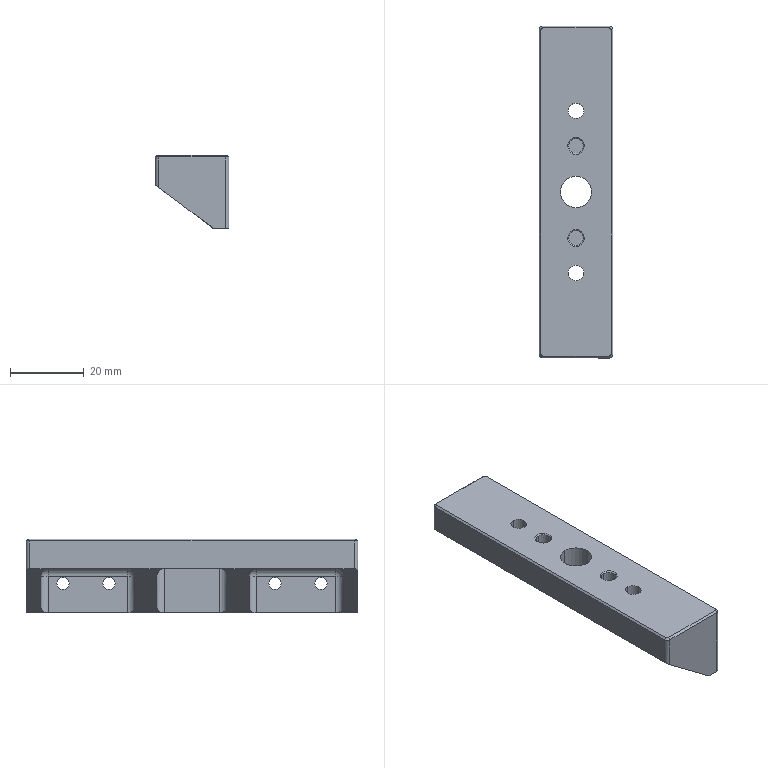NC program | NX | posted with a generic post | part box 20 x 90 x 20 mm
Lines 987 to 2039 of 22268:
(FIXED_CONTOUR , TOOL : D4R0.5)
N1966 T18 M6
N1968 G54
N1970 G17 G0 G90 X37.898 Y-9.972 B0. C0. S9500 M3
N1972 G43 Z30. H18
N1974 Z-7.6
N1976 G94 G1 Z-11.96 F1000.
N1978 X37.887 Y-9.944
N1980 X37.86 Y-9.928
N1982 X37.829 Y-9.932
N1984 X37.745 Z-11.98 F2500.
N1986 X37.579 Z-11.997
N1988 X37.321 Z-12.
N1990 X18.997 Z-11.999
N1992 X18.898 Z-11.996
N1994 X18.751 Z-11.979
N1996 X18.69 Z-11.965
N1998 X18.547 Y-9.858 Z-11.931
N2000 X18.751 Z-11.979
N2002 X18.933 Z-11.998
N2004 X19.144 Z-12.
N2006 X37.53 Y-9.859 Z-11.999
N2008 X37.568 Z-11.998
N2010 X37.745 Z-11.98
N2012 X37.955 Z-11.93
N2014 X37.995 Y-9.835 Z-11.917
N2016 X38.034 Y-9.811 Z-11.9
N2018 X38.082 Y-9.775 Z-11.879
N2020 X37.943 Z-11.933
N2022 X37.745 Z-11.98
N2024 X37.553 Z-11.998
N2026 X37.459 Z-12.
N2028 X19.026
N2030 X18.938 Z-11.998
N2032 X18.751 Z-11.979
N2034 X18.553 Z-11.932
N2036 X18.418 Z-11.879
N2038 X18.356 Y-9.73 Z-11.852
N2040 X18.317 Y-9.702 Z-11.831
N2042 X18.301 Y-9.687 Z-11.822
N2044 X18.355 Z-11.851
N2046 X18.553 Z-11.931
N2048 X18.751 Z-11.978
N2050 X18.949 Z-11.999
N2052 X19.048 Z-12.
N2054 X37.498 Y-9.688
N2056 X37.547 Z-11.998
N2058 X37.745 Z-11.979
N2060 X37.943 Z-11.932
N2062 X38.141 Z-11.854
N2064 X38.194 Z-11.825
N2066 X38.231 Y-9.658 Z-11.805
N2068 X38.288 Y-9.593 Z-11.774
N2070 X38.141 Z-11.853
N2072 X37.943 Z-11.932
N2074 X37.745 Z-11.979
N2076 X37.547 Z-11.998
N2078 X37.498 Z-12.
N2080 X19.048
N2082 X18.949 Z-11.999
N2084 X18.751 Z-11.978
N2086 X18.553 Z-11.931
N2088 X18.355 Z-11.851
N2090 X18.213 Z-11.773
N2092 X18.157 Y-9.529 Z-11.743
N2094 X18.13 Y-9.497 Z-11.725
N2096 X18.157 Z-11.743
N2098 X18.355 Z-11.851
N2100 X18.553 Z-11.931
N2102 X18.751 Z-11.978
N2104 X18.949 Z-11.999
N2106 X19.048 Z-12.
N2108 X37.498
N2110 X37.547 Z-11.998
N2112 X37.745 Z-11.979
N2114 X37.943 Z-11.932
N2116 X38.141 Z-11.853
N2118 X38.339 Z-11.745
N2120 X38.368 Z-11.722
N2122 X38.39 Y-9.468 Z-11.704
N2124 X38.438 Y-9.4 Z-11.665
N2126 X38.339 Z-11.744
N2128 X38.141 Z-11.853
N2130 X37.943 Z-11.932
N2132 X37.745 Z-11.979
N2134 X37.547 Z-11.998
N2136 X37.498 Z-12.
N2138 X19.048
N2140 X18.949 Z-11.999
N2142 X18.751 Z-11.978
N2144 X18.553 Z-11.931
N2146 X18.355 Z-11.851
N2148 X18.157 Z-11.742
N2150 X18.125 Z-11.72
N2152 X18.06 Z-11.668
N2154 X18.017 Y-9.334 Z-11.627
N2156 X17.995 Y-9.303 Z-11.609
N2158 X18.157 Z-11.741
N2160 X18.355 Z-11.851
N2162 X18.553 Z-11.931
N2164 X18.751 Z-11.978
N2166 X18.949 Z-11.999
N2168 X19.048 Z-12.
N2170 X37.498
N2172 X37.547 Z-11.998
N2174 X37.745 Z-11.979
N2176 X37.943 Z-11.932
N2178 X38.141 Z-11.853
N2180 X38.339 Z-11.743
N2182 X38.505 Z-11.61
N2184 X38.537 Y-9.257 Z-11.584
N2186 X38.564 Y-9.205 Z-11.555
N2188 X38.537 Z-11.584
N2190 X38.339 Z-11.743
N2192 X38.141 Z-11.853
N2194 X37.943 Z-11.932
N2196 X37.745 Z-11.979
N2198 X37.547 Z-11.998
N2200 X37.498 Z-12.
N2202 X19.048
N2204 X18.949 Z-11.999
N2206 X18.751 Z-11.978
N2208 X18.553 Z-11.931
N2210 X18.355 Z-11.851
N2212 X18.157 Z-11.741
N2214 X17.96 Z-11.58
N2216 X17.934 Z-11.553
N2218 X17.92 Y-9.178 Z-11.537
N2220 X17.886 Y-9.107 Z-11.499
N2222 X17.96 Z-11.58
N2224 X18.101 Z-11.697
N2226 X18.157 Z-11.741
N2228 X18.355 Z-11.851
N2230 X18.553 Z-11.931
N2232 X18.751 Z-11.978
N2234 X18.949 Z-11.999
N2236 X19.048 Z-12.
N2238 X37.498
N2240 X37.547 Z-11.998
N2242 X37.745 Z-11.979
N2244 X37.943 Z-11.932
N2246 X38.141 Z-11.853
N2248 X38.339 Z-11.743
N2250 X38.396 Z-11.699
N2252 X38.537 Z-11.584
N2254 X38.616 Z-11.498
N2256 X38.664 Y-9.009 Z-11.446
N2258 X38.537 Z-11.584
N2260 X38.42 Z-11.68
N2262 X38.339 Z-11.743
N2264 X38.141 Z-11.853
N2266 X37.943 Z-11.932
N2268 X37.745 Z-11.979
N2270 X37.547 Z-11.998
N2272 X37.498 Z-12.
N2274 X19.048
N2276 X18.949 Z-11.999
N2278 X18.751 Z-11.978
N2280 X18.553 Z-11.931
N2282 X18.355 Z-11.851
N2284 X18.157 Z-11.741
N2286 X18.076 Z-11.678
N2288 X17.96 Z-11.579
N2290 X17.838 Z-11.447
N2292 X17.796 Y-8.91 Z-11.391
N2294 X17.861 Z-11.472
N2296 X17.96 Z-11.579
N2298 X18.059 Z-11.664
N2300 X18.157 Z-11.741
N2302 X18.355 Z-11.851
N2304 X18.553 Z-11.931
N2306 X18.751 Z-11.978
N2308 X18.949 Z-11.999
N2310 X19.048 Z-12.
N2312 X37.498
N2314 X37.547 Z-11.998
N2316 X37.745 Z-11.979
N2318 X37.943 Z-11.932
N2320 X38.141 Z-11.853
N2322 X38.339 Z-11.743
N2324 X38.438 Z-11.667
N2326 X38.537 Z-11.583
N2328 X38.643 Z-11.469
N2330 X38.705 Z-11.388
N2332 X38.745 Y-8.811 Z-11.333
N2334 X38.735 Z-11.349
N2336 X38.636 Z-11.478
N2338 X38.537 Z-11.583
N2340 X38.438 Z-11.667
N2342 X38.339 Z-11.743
N2344 X38.141 Z-11.853
N2346 X37.943 Z-11.932
N2348 X37.745 Z-11.979
N2350 X37.547 Z-11.998
N2352 X37.498 Z-12.
N2354 X19.048
N2356 X18.949 Z-11.999
N2358 X18.751 Z-11.978
N2360 X18.553 Z-11.931
N2362 X18.355 Z-11.851
N2364 X18.157 Z-11.741
N2366 X18.059 Z-11.664
N2368 X17.96 Z-11.579
N2370 X17.861 Z-11.472
N2372 X17.762 Z-11.347
N2374 X17.756 Z-11.337
N2376 X17.722 Y-8.712 Z-11.282
N2378 X17.762 Z-11.347
N2380 X17.861 Z-11.472
N2382 X17.96 Z-11.579
N2384 X18.059 Z-11.664
N2386 X18.157 Z-11.741
N2388 X18.355 Z-11.851
N2390 X18.553 Z-11.931
N2392 X18.751 Z-11.978
N2394 X18.949 Z-11.999
N2396 X19.048 Z-12.
N2398 X37.498
N2400 X37.547 Z-11.998
N2402 X37.745 Z-11.979
N2404 X37.943 Z-11.932
N2406 X38.141 Z-11.853
N2408 X38.339 Z-11.743
N2410 X38.438 Z-11.667
N2412 X38.537 Z-11.583
N2414 X38.636 Z-11.478
N2416 X38.735 Z-11.349
N2418 X38.779 Z-11.276
N2420 X38.811 Y-8.613 Z-11.221
N2422 X38.735 Z-11.349
N2424 X38.636 Z-11.478
N2426 X38.537 Z-11.583
N2428 X38.438 Z-11.667
N2430 X38.339 Z-11.743
N2432 X38.141 Z-11.853
N2434 X37.943 Z-11.932
N2436 X37.745 Z-11.979
N2438 X37.547 Z-11.998
N2440 X37.498 Z-12.
N2442 X19.048
N2444 X18.949 Z-11.999
N2446 X18.751 Z-11.978
N2448 X18.553 Z-11.931
N2450 X18.355 Z-11.851
N2452 X18.157 Z-11.741
N2454 X18.059 Z-11.664
N2456 X17.96 Z-11.579
N2458 X17.861 Z-11.472
N2460 X17.762 Z-11.346
N2462 X17.691 Z-11.225
N2464 X17.66 Y-8.514 Z-11.169
N2466 X17.762 Z-11.346
N2468 X17.861 Z-11.472
N2470 X17.96 Z-11.579
N2472 X18.059 Z-11.664
N2474 X18.157 Z-11.741
N2476 X18.355 Z-11.851
N2478 X18.553 Z-11.931
N2480 X18.751 Z-11.978
N2482 X18.949 Z-11.999
N2484 X19.048 Z-12.
N2486 X37.498 Y-8.515
N2488 X37.547 Z-11.998
N2490 X37.745 Z-11.979
N2492 X37.943 Z-11.932
N2494 X38.141 Z-11.853
N2496 X38.339 Z-11.743
N2498 X38.438 Z-11.667
N2500 X38.537 Z-11.583
N2502 X38.636 Z-11.478
N2504 X38.735 Z-11.349
N2506 X38.841 Z-11.166
N2508 X38.869 Y-8.416 Z-11.113
N2510 X38.834 Z-11.181
N2512 X38.735 Z-11.349
N2514 X38.636 Z-11.478
N2516 X38.537 Z-11.583
N2518 X38.438 Z-11.667
N2520 X38.339 Z-11.743
N2522 X38.141 Z-11.853
N2524 X37.943 Z-11.932
N2526 X37.745 Z-11.979
N2528 X37.547 Z-11.998
N2530 X37.498 Z-12.
N2532 X19.048 Y-8.415
N2534 X18.949 Z-11.999
N2536 X18.751 Z-11.978
N2538 X18.553 Z-11.931
N2540 X18.355 Z-11.851
N2542 X18.157 Z-11.741
N2544 X18.059 Z-11.664
N2546 X17.96 Z-11.579
N2548 X17.861 Z-11.472
N2550 X17.762 Z-11.346
N2552 X17.663 Z-11.174
N2554 X17.632 Z-11.114
N2556 X17.605 Y-8.316 Z-11.061
N2558 X17.635 Z-11.115
N2560 X17.663 Z-11.174
N2562 X17.762 Z-11.346
N2564 X17.861 Z-11.472
N2566 X17.96 Z-11.579
N2568 X18.059 Z-11.664
N2570 X18.157 Z-11.741
N2572 X18.355 Z-11.851
N2574 X18.553 Z-11.931
N2576 X18.751 Z-11.978
N2578 X18.949 Z-11.999
N2580 X19.048 Z-12.
N2582 X37.498
N2584 X37.547 Z-11.998
N2586 X37.745 Z-11.979
N2588 X37.943 Z-11.932
N2590 X38.141 Z-11.853
N2592 X38.339 Z-11.743
N2594 X38.438 Z-11.667
N2596 X38.537 Z-11.583
N2598 X38.636 Z-11.478
N2600 X38.735 Z-11.349
N2602 X38.834 Z-11.181
N2604 X38.862 Z-11.123
N2606 X38.896 Z-11.06
N2608 X38.902 Y-8.296 Z-11.049
N2610 X38.913 Y-8.218 Z-11.002
N2612 X38.892 Z-11.065
N2614 X38.834 Z-11.181
N2616 X38.735 Z-11.349
N2618 X38.636 Z-11.478
N2620 X38.537 Z-11.583
N2622 X38.438 Z-11.667
N2624 X38.339 Z-11.743
N2626 X38.141 Z-11.853
N2628 X37.943 Z-11.932
N2630 X37.745 Z-11.979
N2632 X37.547 Z-11.998
N2634 X37.498 Z-12.
N2636 X19.048
N2638 X18.949 Z-11.999
N2640 X18.751 Z-11.978
N2642 X18.553 Z-11.931
N2644 X18.355 Z-11.851
N2646 X18.157 Z-11.741
N2648 X18.059 Z-11.664
N2650 X17.96 Z-11.579
N2652 X17.861 Z-11.472
N2654 X17.762 Z-11.346
N2656 X17.663 Z-11.174
N2658 X17.622 Z-11.089
N2660 X17.604 Z-11.056
N2662 X17.587 Z-11.002
N2664 X17.571 Y-8.118 Z-10.944
N2666 X17.613 Z-11.071
N2668 X17.663 Z-11.174
N2670 X17.762 Z-11.346
N2672 X17.861 Z-11.472
N2674 X17.96 Z-11.579
N2676 X18.059 Z-11.664
N2678 X18.157 Z-11.741
N2680 X18.355 Z-11.851
N2682 X18.553 Z-11.931
N2684 X18.751 Z-11.978
N2686 X18.949 Z-11.999
N2688 X19.048 Z-12.
N2690 X37.498 Y-8.119
N2692 X37.547 Z-11.998
N2694 X37.745 Z-11.979
N2696 X37.943 Z-11.931
N2698 X38.141 Z-11.853
N2700 X38.339 Z-11.743
N2702 X38.438 Z-11.667
N2704 X38.537 Z-11.583
N2706 X38.636 Z-11.478
N2708 X38.735 Z-11.349
N2710 X38.834 Z-11.181
N2712 X38.883 Z-11.079
N2714 X38.93 Z-10.945
N2716 X38.949 Y-8.019 Z-10.888
N2718 X38.883 Z-11.079
N2720 X38.834 Z-11.181
N2722 X38.735 Z-11.349
N2724 X38.636 Z-11.478
N2726 X38.537 Z-11.583
N2728 X38.438 Z-11.667
N2730 X38.339 Z-11.743
N2732 X38.141 Z-11.853
N2734 X37.943 Z-11.931
N2736 X37.745 Z-11.979
N2738 X37.547 Z-11.998
N2740 X37.498 Z-12.
N2742 X19.048
N2744 X18.949 Z-11.999
N2746 X18.751 Z-11.978
N2748 X18.553 Z-11.931
N2750 X18.355 Z-11.851
N2752 X18.157 Z-11.741
N2754 X18.059 Z-11.664
N2756 X17.96 Z-11.579
N2758 X17.861 Z-11.472
N2760 X17.762 Z-11.345
N2762 X17.663 Z-11.174
N2764 X17.613 Z-11.071
N2766 X17.564 Z-10.924
N2768 X17.555 Z-10.888
N2770 X17.541 Y-7.92 Z-10.832
N2772 X17.564 Z-10.923
N2774 X17.613 Z-11.071
N2776 X17.663 Z-11.174
N2778 X17.762 Z-11.345
N2780 X17.861 Z-11.472
N2782 X17.96 Z-11.579
N2784 X18.059 Z-11.663
N2786 X18.157 Z-11.741
N2788 X18.355 Z-11.851
N2790 X18.553 Z-11.931
N2792 X18.751 Z-11.978
N2794 X18.949 Z-11.999
N2796 X19.048 Z-12.
N2798 X37.498
N2800 X37.547 Z-11.998
N2802 X37.745 Z-11.978
N2804 X37.943 Z-11.931
N2806 X38.141 Z-11.853
N2808 X38.339 Z-11.743
N2810 X38.438 Z-11.667
N2812 X38.537 Z-11.583
N2814 X38.636 Z-11.478
N2816 X38.735 Z-11.349
N2818 X38.834 Z-11.181
N2820 X38.883 Z-11.079
N2822 X38.954 Z-10.874
N2824 X38.963 Z-10.829
N2826 X38.972 Y-7.82 Z-10.769
N2828 X38.941 Z-10.91
N2830 X38.883 Z-11.079
N2832 X38.834 Z-11.181
N2834 X38.735 Z-11.349
N2836 X38.636 Z-11.478
N2838 X38.537 Z-11.583
N2840 X38.438 Z-11.667
N2842 X38.339 Z-11.743
N2844 X38.141 Z-11.853
N2846 X37.943 Z-11.931
N2848 X37.745 Z-11.978
N2850 X37.547 Z-11.998
N2852 X37.498 Z-12.
N2854 X19.048
N2856 X18.949 Z-11.999
N2858 X18.751 Z-11.978
N2860 X18.553 Z-11.931
N2862 X18.355 Z-11.851
N2864 X18.157 Z-11.741
N2866 X18.059 Z-11.663
N2868 X17.96 Z-11.579
N2870 X17.861 Z-11.472
N2872 X17.762 Z-11.345
N2874 X17.663 Z-11.174
N2876 X17.613 Z-11.071
N2878 X17.564 Z-10.923
N2880 X17.53 Z-10.775
N2882 X17.518 Y-7.72 Z-10.718
N2884 X17.564 Z-10.923
N2886 X17.613 Z-11.071
N2888 X17.663 Z-11.174
N2890 X17.762 Z-11.345
N2892 X17.861 Z-11.472
N2894 X17.96 Z-11.579
N2896 X18.059 Z-11.663
N2898 X18.157 Z-11.741
N2900 X18.355 Z-11.851
N2902 X18.553 Z-11.931
N2904 X18.751 Z-11.978
N2906 X18.949 Z-11.999
N2908 X19.048 Z-12.
N2910 X37.498 Y-7.721
N2912 X37.547 Z-11.998
N2914 X37.745 Z-11.978
N2916 X37.943 Z-11.931
N2918 X38.141 Z-11.853
N2920 X38.339 Z-11.743
N2922 X38.438 Z-11.667
N2924 X38.537 Z-11.583
N2926 X38.636 Z-11.478
N2928 X38.735 Z-11.349
N2930 X38.834 Z-11.181
N2932 X38.883 Z-11.079
N2934 X38.933 Z-10.935
N2936 X38.982 Z-10.709
N2938 X38.985 Y-7.681 Z-10.684
N2940 X38.988 Y-7.622 Z-10.643
N2942 X38.982 Z-10.707
N2944 X38.933 Z-10.935
N2946 X38.883 Z-11.079
N2948 X38.834 Z-11.181
N2950 X38.735 Z-11.349
N2952 X38.636 Z-11.478
N2954 X38.537 Z-11.583
N2956 X38.438 Z-11.667
N2958 X38.339 Y-7.621 Z-11.743
N2960 X38.141 Z-11.853
N2962 X37.943 Z-11.931
N2964 X37.745 Z-11.978
N2966 X37.547 Z-11.998
N2968 X37.498 Z-12.
N2970 X19.048
N2972 X18.949 Z-11.999
N2974 X18.751 Z-11.978
N2976 X18.553 Z-11.931
N2978 X18.355 Z-11.851
N2980 X18.157 Z-11.741
N2982 X18.059 Z-11.663
N2984 X17.96 Z-11.579
N2986 X17.861 Z-11.472
N2988 X17.762 Z-11.345
N2990 X17.663 Z-11.174
N2992 X17.613 Z-11.071
N2994 X17.564 Z-10.923
N2996 X17.514 Z-10.703
N2998 X17.511 Z-10.664
N3000 X17.507 Y-7.522 Z-10.61
N3002 X17.514 Z-10.703
N3004 X17.564 Z-10.923
N3006 X17.613 Z-11.071
N3008 X17.663 Z-11.174
N3010 X17.762 Z-11.345
N3012 X17.861 Z-11.472
N3014 X17.96 Z-11.579
N3016 X18.059 Z-11.663
N3018 X18.157 Z-11.741
N3020 X18.355 Z-11.851
N3022 X18.553 Z-11.931
N3024 X18.751 Z-11.978
N3026 X18.949 Z-11.999
N3028 X19.048 Z-12.
N3030 X37.498
N3032 X37.547 Z-11.998
N3034 X37.745 Z-11.978
N3036 X37.943 Z-11.931
N3038 X38.141 Z-11.853
N3040 X38.339 Z-11.743
N3042 X38.438 Z-11.667
N3044 X38.537 Z-11.582
N3046 X38.636 Z-11.478
N3048 X38.735 Z-11.349
N3050 X38.834 Z-11.181
N3052 X38.883 Z-11.079
N3054 X38.933 Z-10.935
N3056 X38.982 Z-10.705
N3058 X38.991 Z-10.63
N3060 X38.993 Z-10.573
N3062 X38.998 Y-7.423 Z-10.504
N3064 X38.992 Z-10.625
N3066 X38.982 Z-10.704
N3068 X38.933 Z-10.935
N3070 X38.883 Z-11.079
N3072 X38.834 Z-11.181
N3074 X38.735 Z-11.349
N3076 X38.636 Z-11.478
N3078 X38.537 Z-11.582
N3080 X38.438 Z-11.667
N3082 X38.339 Z-11.743
N3084 X38.141 Z-11.853
N3086 X37.943 Z-11.931
N3088 X37.745 Z-11.978
N3090 X37.547 Z-11.998
N3092 X37.498 Z-12.
N3094 X19.048 Y-7.422
N3096 X18.949 Z-11.999
N3098 X18.751 Z-11.978
N3100 X18.553 Z-11.931
N3102 X18.355 Z-11.851
N3104 X18.157 Z-11.741
N3106 X18.059 Z-11.663
N3108 X17.96 Z-11.579
N3110 X17.861 Z-11.472
N3112 X17.762 Z-11.345
N3114 X17.663 Z-11.174
N3116 X17.613 Z-11.071
N3118 X17.564 Z-10.923
N3120 X17.514 Z-10.703
N3122 X17.504 Z-10.556
N3124 X17.501 Y-7.323 Z-10.502
N3126 X17.502 Z-10.544
N3128 X17.516 Z-10.711
N3130 X17.564 Z-10.923
N3132 X17.613 Z-11.071
N3134 X17.663 Z-11.174
N3136 X17.762 Z-11.345
N3138 X17.861 Z-11.472
N3140 X17.96 Z-11.579
N3142 X18.059 Z-11.663
N3144 X18.157 Z-11.741
N3146 X18.355 Z-11.851
N3148 X18.553 Z-11.931
N3150 X18.751 Z-11.978
N3152 X18.949 Z-11.999
N3154 X19.048 Z-12.
N3156 X37.498
N3158 X37.547 Z-11.998
N3160 X37.745 Z-11.978
N3162 X37.943 Z-11.931
N3164 X38.141 Z-11.853
N3166 X38.339 Z-11.743
N3168 X38.438 Z-11.667
N3170 X38.537 Z-11.582
N3172 X38.636 Z-11.478
N3174 X38.735 Z-11.349
N3176 X38.834 Z-11.181
N3178 X38.883 Z-11.079
N3180 X38.933 Z-10.935
N3182 X38.982 Z-10.704
N3184 X38.997 Z-10.574
N3186 X39.002 Z-10.434
N3188 X39.001 Y-7.223 Z-10.36
N3190 X38.997 Z-10.579
N3192 X38.982 Z-10.704
N3194 X38.933 Z-10.935
N3196 X38.883 Z-11.079
N3198 X38.834 Z-11.181
N3200 X38.735 Z-11.349
N3202 X38.636 Z-11.478
N3204 X38.537 Z-11.582
N3206 X38.438 Z-11.667
N3208 X38.339 Z-11.743
N3210 X38.141 Z-11.853
N3212 X37.943 Z-11.931
N3214 X37.745 Z-11.978
N3216 X37.547 Z-11.998
N3218 X37.498 Z-12.
N3220 X19.048
N3222 X18.949 Z-11.999
N3224 X18.751 Z-11.978
N3226 X18.553 Z-11.931
N3228 X18.355 Z-11.851
N3230 X18.157 Z-11.741
N3232 X18.059 Z-11.663
N3234 X17.96 Z-11.579
N3236 X17.861 Z-11.472
N3238 X17.762 Z-11.345
N3240 X17.663 Z-11.174
N3242 X17.613 Z-11.071
N3244 X17.564 Z-10.923
N3246 X17.516 Z-10.71
N3248 X17.501 Z-10.523
N3250 Z-10.426
N3252 Y-7.124 Z-10.344
N3254 X17.503 Z-10.554
N3256 X17.517 Z-10.715
N3258 X17.546 Z-10.851
N3260 X17.564 Z-10.923
N3262 X17.613 Z-11.071
N3264 X17.663 Z-11.174
N3266 X17.762 Z-11.345
N3268 X17.861 Z-11.472
N3270 X17.96 Z-11.579
N3272 X18.059 Z-11.663
N3274 X18.157 Z-11.741
N3276 X18.355 Z-11.851
N3278 X18.553 Z-11.931
N3280 X18.751 Z-11.978
N3282 X18.949 Z-11.999
N3284 X19.048 Z-12.
N3286 X37.498
N3288 X37.547 Z-11.998
N3290 X37.745 Z-11.978
N3292 X37.943 Z-11.931
N3294 X38.141 Z-11.853
N3296 X38.339 Z-11.743
N3298 X38.438 Z-11.667
N3300 X38.537 Z-11.582
N3302 X38.636 Z-11.478
N3304 X38.735 Z-11.349
N3306 X38.834 Z-11.181
N3308 X38.883 Z-11.079
N3310 X38.933 Z-10.935
N3312 X38.982 Z-10.704
N3314 X38.997 Z-10.583
N3316 X39.001 Z-10.286
N3318 Y-7.025 Z-10.212
N3320 X38.996 Z-10.593
N3322 X38.982 Z-10.704
N3324 X38.933 Z-10.935
N3326 X38.883 Z-11.079
N3328 X38.834 Z-11.181
N3330 X38.735 Z-11.349
N3332 X38.636 Z-11.478
N3334 X38.537 Z-11.582
N3336 X38.438 Z-11.667
N3338 X38.339 Z-11.743
N3340 X38.141 Z-11.853
N3342 X37.943 Z-11.931
N3344 X37.745 Z-11.978
N3346 X37.547 Z-11.998
N3348 X37.498 Z-12.
N3350 X19.048
N3352 X18.949 Z-11.999
N3354 X18.751 Z-11.978
N3356 X18.553 Z-11.931
N3358 X18.355 Z-11.851
N3360 X18.157 Z-11.741
N3362 X18.059 Z-11.663
N3364 X17.96 Z-11.579
N3366 X17.861 Z-11.473
N3368 X17.762 Z-11.345
N3370 X17.663 Z-11.174
N3372 X17.613 Z-11.071
N3374 X17.564 Z-10.923
N3376 X17.53 Z-10.782
N3378 X17.518 Z-10.72
N3380 X17.503 Z-10.549
N3382 X17.501 Z-10.264
N3384 Y-6.928 Z-10.184
N3386 X17.504 Z-10.574
N3388 X17.518 Z-10.721
N3390 X17.536 Z-10.808
N3392 X17.564 Z-10.923
N3394 X17.613 Z-11.071
N3396 X17.663 Z-11.174
N3398 X17.762 Z-11.345
N3400 X17.861 Z-11.473
N3402 X17.96 Z-11.578
N3404 X18.059 Z-11.663
N3406 X18.157 Z-11.741
N3408 X18.355 Z-11.851
N3410 X18.553 Z-11.931
N3412 X18.751 Z-11.977
N3414 X18.949 Z-11.999
N3416 X19.048 Z-12.
N3418 X37.498
N3420 X37.547 Z-11.998
N3422 X37.745 Z-11.978
N3424 X37.943 Z-11.931
N3426 X38.141 Z-11.853
N3428 X38.339 Z-11.743
N3430 X38.438 Z-11.667
N3432 X38.537 Z-11.582
N3434 X38.636 Z-11.478
N3436 X38.735 Z-11.349
N3438 X38.834 Z-11.181
N3440 X38.883 Z-11.079
N3442 X38.933 Z-10.935
N3444 X38.982 Z-10.704
N3446 X38.997 Z-10.59
N3448 X39.001 Z-10.139
N3450 Y-6.831 Z-10.066
N3452 X38.997 Z-10.59
N3454 X38.982 Z-10.703
N3456 X38.933 Z-10.935
N3458 X38.883 Z-11.079
N3460 X38.834 Z-11.181
N3462 X38.735 Z-11.349
N3464 X38.636 Z-11.478
N3466 X38.537 Z-11.582
N3468 X38.438 Z-11.667
N3470 X38.339 Z-11.743
N3472 X38.141 Z-11.853
N3474 X37.943 Z-11.931
N3476 X37.745 Z-11.978
N3478 X37.547 Z-11.998
N3480 X37.498 Z-12.
N3482 X19.048 Y-6.83
N3484 X18.949 Z-11.999
N3486 X18.751 Z-11.977
N3488 X18.553 Z-11.931
N3490 X18.355 Z-11.851
N3492 X18.157 Z-11.741
N3494 X18.059 Z-11.663
N3496 X17.96 Z-11.578
N3498 X17.861 Z-11.473
N3500 X17.762 Z-11.345
N3502 X17.663 Z-11.174
N3504 X17.613 Z-11.071
N3506 X17.564 Z-10.923
N3508 X17.527 Z-10.766
N3510 X17.517 Z-10.715
N3512 X17.502 Z-10.543
N3514 X17.5 Z-10.109
N3516 Y-6.733 Z-10.036
N3518 X17.502 Z-10.549
N3520 X17.516 Z-10.71
N3522 X17.564 Z-10.923
N3524 X17.613 Z-11.071
N3526 X17.663 Z-11.174
N3528 X17.762 Z-11.344
N3530 X17.861 Z-11.473
N3532 X17.96 Z-11.578
N3534 X18.059 Z-11.663
N3536 X18.157 Z-11.741
N3538 X18.355 Z-11.851
N3540 X18.553 Z-11.931
N3542 X18.751 Z-11.977
N3544 X18.949 Z-11.999
N3546 X19.048 Z-12.
N3548 X37.498
N3550 X37.547 Z-11.998
N3552 X37.745 Z-11.978
N3554 X37.943 Z-11.931
N3556 X38.141 Z-11.853
N3558 X38.339 Z-11.743
N3560 X38.438 Z-11.667
N3562 X38.537 Z-11.582
N3564 X38.636 Z-11.478
N3566 X38.735 Z-11.349
N3568 X38.834 Z-11.181
N3570 X38.883 Z-11.078
N3572 X38.933 Z-10.936
N3574 X38.982 Z-10.703
N3576 X38.997 Z-10.59
N3578 X39.001 Z-9.993
N3580 Y-6.636 Z-9.92
N3582 X38.997 Z-10.59
N3584 X38.982 Z-10.703
N3586 X38.933 Z-10.936
N3588 X38.883 Z-11.078
N3590 X38.834 Z-11.181
N3592 X38.735 Z-11.349
N3594 X38.636 Z-11.478
N3596 X38.537 Z-11.582
N3598 X38.438 Z-11.667
N3600 X38.339 Z-11.743
N3602 X38.141 Z-11.853
N3604 X37.943 Z-11.931
N3606 X37.745 Z-11.978
N3608 X37.547 Z-11.998
N3610 X37.498 Z-12.
N3612 X19.048
N3614 X18.949 Z-11.999
N3616 X18.751 Z-11.977
N3618 X18.553 Z-11.931
N3620 X18.355 Z-11.851
N3622 X18.157 Z-11.741
N3624 X18.059 Z-11.663
N3626 X17.96 Z-11.578
N3628 X17.861 Z-11.473
N3630 X17.762 Z-11.344
N3632 X17.663 Z-11.174
N3634 X17.613 Z-11.071
N3636 X17.564 Z-10.923
N3638 X17.515 Z-10.704
N3640 X17.501 Z-10.511
N3642 X17.499 Z-9.963
N3644 Y-6.538 Z-9.89
N3646 X17.501 Z-10.5
N3648 X17.514 Z-10.699
N3650 X17.564 Z-10.923
N3652 X17.613 Z-11.071
N3654 X17.663 Z-11.174
N3656 X17.762 Z-11.344
N3658 X17.861 Z-11.473
N3660 X17.96 Z-11.578
N3662 X18.059 Z-11.663
N3664 X18.157 Z-11.741
N3666 X18.355 Z-11.851
N3668 X18.553 Z-11.931
N3670 X18.751 Z-11.977
N3672 X18.949 Z-11.999
N3674 X19.042 Z-12.
N3676 X37.498 Y-6.539
N3678 X37.547 Z-11.998
N3680 X37.745 Z-11.978
N3682 X37.943 Z-11.931
N3684 X38.141 Z-11.853
N3686 X38.339 Z-11.743
N3688 X38.438 Z-11.668
N3690 X38.537 Z-11.582
N3692 X38.636 Z-11.478
N3694 X38.735 Z-11.349
N3696 X38.834 Z-11.181
N3698 X38.883 Z-11.078
N3700 X38.933 Z-10.936
N3702 X38.982 Z-10.703
N3704 X38.997 Z-10.59
N3706 X39.001 Z-9.847
N3708 Y-6.441 Z-9.774
N3710 X38.997 Z-10.59
N3712 X38.982 Z-10.703
N3714 X38.933 Z-10.936
N3716 X38.883 Z-11.078
N3718 X38.834 Z-11.18
N3720 X38.735 Z-11.349
N3722 X38.636 Z-11.478
N3724 X38.537 Z-11.582
N3726 X38.438 Z-11.668
N3728 X38.339 Z-11.743
N3730 X38.141 Z-11.853
N3732 X37.943 Z-11.931
N3734 X37.745 Z-11.978
N3736 X37.547 Z-11.998
N3738 X37.498 Z-12.
N3740 X19.048
N3742 X18.949 Z-11.998
N3744 X18.751 Z-11.977
N3746 X18.553 Z-11.931
N3748 X18.355 Z-11.851
N3750 X18.157 Z-11.741
N3752 X18.059 Z-11.663
N3754 X17.96 Z-11.578
N3756 X17.861 Z-11.473
N3758 X17.762 Z-11.344
N3760 X17.663 Z-11.174
N3762 X17.613 Z-11.071
N3764 X17.564 Z-10.923
N3766 X17.514 Z-10.699
N3768 X17.501 Z-10.499
N3770 X17.499 Z-9.817
N3772 Y-6.344 Z-9.744
N3774 X17.501 Z-10.499
N3776 X17.514 Z-10.698
N3778 X17.564 Z-10.923
N3780 X17.613 Z-11.071
N3782 X17.663 Z-11.174
N3784 X17.762 Z-11.344
N3786 X17.861 Z-11.473
N3788 X17.96 Z-11.578
N3790 X18.059 Z-11.663
N3792 X18.157 Z-11.741
N3794 X18.355 Z-11.851
N3796 X18.553 Z-11.931
N3798 X18.751 Z-11.977
N3800 X18.949 Z-11.998
N3802 X19.048 Z-12.
N3804 X37.498
N3806 X37.547 Z-11.998
N3808 X37.745 Z-11.978
N3810 X37.943 Z-11.931
N3812 X38.141 Z-11.853
N3814 X38.339 Z-11.743
N3816 X38.438 Z-11.668
N3818 X38.537 Z-11.582
N3820 X38.636 Z-11.478
N3822 X38.735 Z-11.349
N3824 X38.834 Z-11.18
N3826 X38.883 Z-11.078
N3828 X38.933 Z-10.936
N3830 X38.982 Z-10.703
N3832 X38.997 Z-10.59
N3834 X39.001 Z-9.701
N3836 Y-6.246 Z-9.628
N3838 X38.997 Z-10.59
N3840 X38.982 Z-10.703
N3842 X38.933 Z-10.936
N3844 X38.883 Z-11.078
N3846 X38.834 Z-11.18
N3848 X38.735 Z-11.349
N3850 X38.636 Z-11.478
N3852 X38.537 Z-11.582
N3854 X38.438 Z-11.668
N3856 X38.339 Z-11.743
N3858 X38.141 Z-11.853
N3860 X37.943 Z-11.931
N3862 X37.745 Z-11.978
N3864 X37.547 Z-11.998
N3866 X37.498 Z-12.
N3868 X19.048
N3870 X18.949 Z-11.998
N3872 X18.751 Z-11.977
N3874 X18.553 Z-11.931
N3876 X18.355 Z-11.851
N3878 X18.157 Z-11.741
N3880 X18.059 Z-11.663
N3882 X17.96 Z-11.578
N3884 X17.861 Z-11.473
N3886 X17.762 Z-11.344
N3888 X17.663 Z-11.174
N3890 X17.613 Z-11.071
N3892 X17.564 Z-10.923
N3894 X17.514 Z-10.698
N3896 X17.501 Z-10.498
N3898 X17.5 Z-9.67
N3900 Y-6.149 Z-9.597
N3902 X17.501 Z-10.498
N3904 X17.514 Z-10.697
N3906 X17.564 Z-10.923
N3908 X17.613 Z-11.071
N3910 X17.663 Z-11.174
N3912 X17.762 Z-11.344
N3914 X17.861 Z-11.473
N3916 X17.96 Z-11.578
N3918 X18.059 Z-11.663
N3920 X18.157 Z-11.741
N3922 X18.355 Z-11.851
N3924 X18.553 Z-11.931
N3926 X18.751 Z-11.977
N3928 X18.949 Z-11.998
N3930 X19.043 Z-12.
N3932 X37.498
N3934 X37.547 Z-11.998
N3936 X37.745 Z-11.978
N3938 X37.943 Z-11.931
N3940 X38.141 Z-11.853
N3942 X38.339 Z-11.743
N3944 X38.438 Z-11.668
N3946 X38.537 Z-11.582
N3948 X38.636 Z-11.478
N3950 X38.735 Z-11.349
N3952 X38.834 Z-11.18
N3954 X38.883 Z-11.078
N3956 X38.933 Z-10.936
N3958 X38.982 Z-10.703
N3960 X38.996 Z-10.591
N3962 X39.001 Z-9.555
N3964 Y-6.052 Z-9.482
N3966 X38.997 Z-10.589
N3968 X38.982 Z-10.703
N3970 X38.933 Z-10.936
N3972 X38.883 Z-11.078
N3974 X38.834 Z-11.18
N3976 X38.735 Z-11.349
N3978 X38.636 Z-11.478
N3980 X38.537 Z-11.582
N3982 X38.438 Z-11.668
N3984 X38.339 Z-11.743
N3986 X38.141 Z-11.853
N3988 X37.943 Z-11.931
N3990 X37.745 Z-11.978
N3992 X37.547 Z-11.998
N3994 X37.498 Z-12.
N3996 X19.048 Y-6.051
N3998 X18.949 Z-11.998
N4000 X18.751 Z-11.977
N4002 X18.553 Z-11.931
N4004 X18.355 Z-11.851
N4006 X18.157 Z-11.741
N4008 X18.059 Z-11.663
N4010 X17.96 Z-11.578
N4012 X17.861 Z-11.473
N4014 X17.762 Z-11.344
N4016 X17.663 Z-11.175
N4018 X17.613 Z-11.071
N4020 X17.564 Z-10.922
N4022 X17.514 Z-10.697
N4024 X17.501 Z-10.498
N4026 X17.5 Z-9.524
N4028 Y-5.954 Z-9.451
N4030 X17.501 Z-10.498
N4032 X17.514 Z-10.696
N4034 X17.564 Z-10.922
N4036 X17.613 Z-11.071
N4038 X17.663 Z-11.175
N4040 X17.762 Z-11.344
N4042 X17.861 Z-11.473
N4044 X17.96 Z-11.578
N4046 X18.059 Z-11.663
N4048 X18.157 Z-11.741
N4050 X18.355 Z-11.851
N4052 X18.553 Z-11.931
N4054 X18.751 Z-11.977
N4056 X18.949 Z-11.998
N4058 X19.048 Z-12.
N4060 X37.498
N4062 X37.547 Z-11.998
N4064 X37.745 Z-11.977